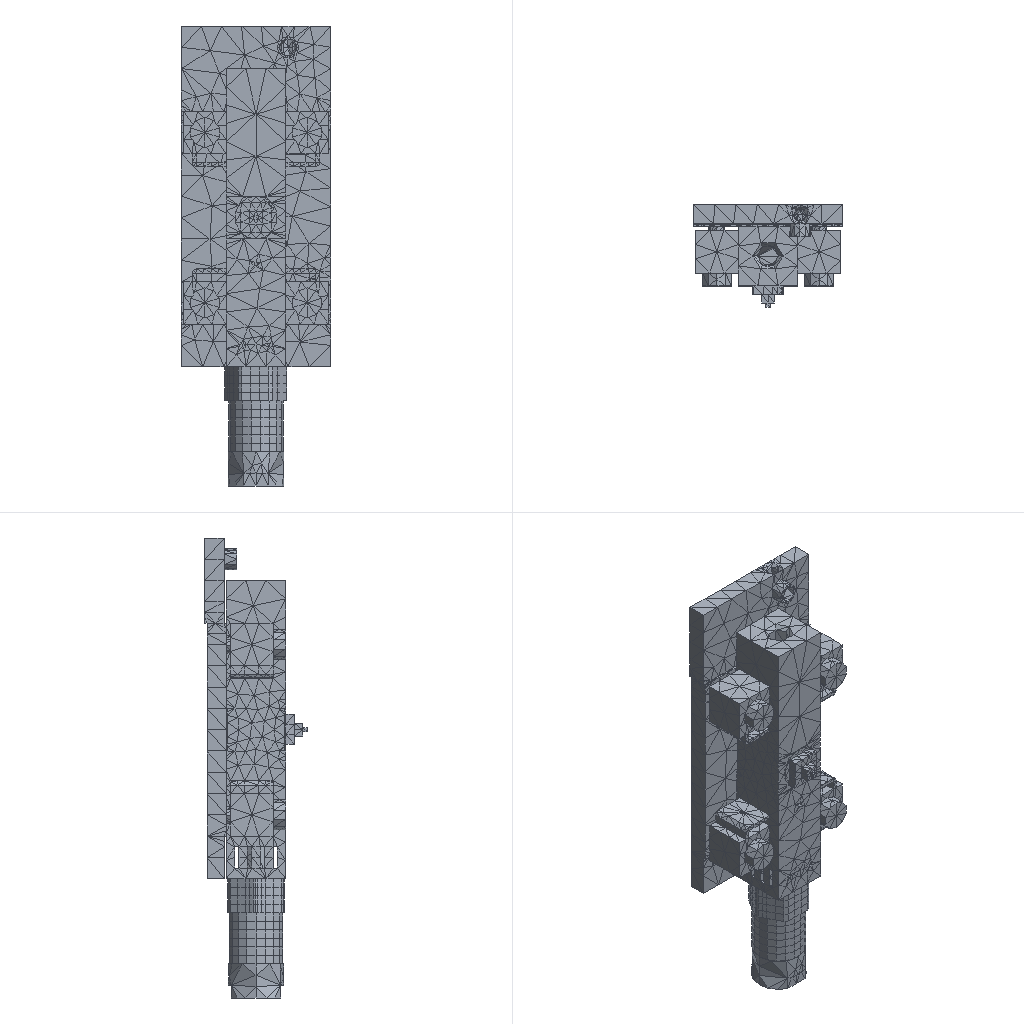Simulation study | ansys workbench
Ansys APDL input file, long lists of numbers shortened:
/batch
/config,noeldb,1     ! force off writing results to database
*get,_wallstrt,active,,time,wall
! ANSYS input file written by Workbench version 2022 R1
! File used for geometry attach: F:\ansys（分析文件汇总)\含底座模态分析\新建文件夹(4)\新建文件夹\完整版.STEP
/title,11111--__ (B5)
! ****** Begin Custom Load Command Snippet ******
/COM, ACT Extensions:
/COM,     LSDYNA, 2021.1
/COM,
! ****** End   Custom Load Command Snippet ******
*DIM,_wb_ProjectScratch_dir,string,248
_wb_ProjectScratch_dir(1) = 'F:\ansys（分析文件汇总)\含底座模态分析\_ProjectScratch\ScrD5D2\'
*DIM,_wb_SolverFiles_dir,string,248
_wb_SolverFiles_dir(1) = 'F:\ansys（分析文件汇总)\含底座模态分析\11111_files\dp0\SYS\MECH\'
*DIM,_wb_userfiles_dir,string,248
_wb_userfiles_dir(1) = 'F:\ansys（分析文件汇总)\含底座模态分析\11111_files\user_files\'
/com,--- Data in consistent NMM units. See Solving Units in the help system for more information.
/units,MPA
/nopr
/wb,file,start              !  signify a WB generated input file
/prep7
! Turn off shape checking because checks already performed inside WB mesher.
! See help system for more information.
SHPP,OFF,,NOWARN
/nolist
etcon,set             ! allow ANSYS to choose best KEYOP's for 180x elements, resets any applicable keyopt to MAPDL defaults
/com,*********** Nodes for the whole assembly ***********
nblock,3,,23060
(1i9,3e20.9e3)
        1    -7.593879241E+01     6.122424365E-01     1.555868903E+01
! (20963 more lines like these left out)
-1
/wb,elem,start            !  set before creation of elements
/com,*********** Elements for Body 1 "__|__-__6" ***********
et,1,187
eblock,19,solid,,4865
(19i9)
        1        1        1        1        0        0        0        0       10        0     2024     8034     8303     8491     8312    14700    15906    14703    14701
! (9729 more lines like these left out)
-1
/com,*********** Elements for Body 2 "___|__-__1" ***********
et,2,186
keyo,2,2,1          ! set full integration on SOLID186
eblock,19,solid,,35
(19i9)
        2        2        2        2        0        0        0        0       20        0      840     2544     2556     2561     2557     2579     2567     2562     2566
! (69 more lines like these left out)
-1
/com,*********** Elements for Body 3 "___|__-__1[2]" ***********
et,3,186
keyo,3,2,1          ! set full integration on SOLID186
eblock,19,solid,,35
(19i9)
        3        3        3        3        0        0        0        0       20        0      770     1924     1936     1941     1937     1959     1947     1942     1946
! (69 more lines like these left out)
-1
/com,*********** Elements for Body 4 "___|__-__1[3]" ***********
et,4,186
keyo,4,2,1          ! set full integration on SOLID186
eblock,19,solid,,35
(19i9)
        4        4        4        4        0        0        0        0       20        0      910     3164     3176     3181     3177     3199     3187     3182     3186
! (69 more lines like these left out)
-1
/com,*********** Elements for Body 5 "___|__-__1[4]" ***********
et,5,186
keyo,5,2,1          ! set full integration on SOLID186
eblock,19,solid,,35
(19i9)
        5        5        5        5        0        0        0        0       20        0      805     2234     2246     2251     2247     2269     2257     2252     2256
! (69 more lines like these left out)
-1
! (11 more sections like these left out)
/wb,elem,end               !  done creating elements
/com,*********** Send User Defined Coordinate System(s) ***********
csys,0
toffst,273.15,  ! Temperature offset from absolute zero
/com,*********** Set Reference Temperature ***********
tref,22.
/wb,mat,start              !  starting to send materials
/com,*********** Send Materials ***********
Temperature = 'TEMP' ! Temperature
TB,BISO,1,5,
TBTEMP,100
TBDATA,1,225,2091
TBTEMP,300
TBDATA,1,168,1577
TBTEMP,816
TBDATA,1,115,708
TBTEMP,1040
TBDATA,1,31,405
TBTEMP,1150
TBDATA,1,15,265
MPTEMP,,,,,,,,
MPTEMP,1,20
MPTEMP,2,100
MPTEMP,3,200
MPTEMP,4,300
MPTEMP,5,400
MPTEMP,6,500
MPTEMP,7,600
MPTEMP,8,700
MPTEMP,9,800
MPTEMP,10,900
MPTEMP,11,1000
MPTEMP,12,1100
MPTEMP,13,1200
MPDATA,EX,1, ,195000,191000,186000,180000,173000,164000,
MPDATA,EX,1, ,155000,144000,131000,117000,100000,81000,
MPDATA,EX,1, ,51000,	! tonne s^-2 mm^-1
MPTEMP,,,,,,,,
MPTEMP,,,,,,,,
MPTEMP,1,20
MPTEMP,2,100
MPTEMP,3,200
MPTEMP,4,300
MPTEMP,5,400
MPTEMP,6,500
MPTEMP,7,600
MPTEMP,8,700
MPTEMP,9,800
MPTEMP,10,900
MPTEMP,11,1000
MPTEMP,12,1100
MPTEMP,13,1200
MPDATA,NUXY,1, ,0.25,0.26,0.275,0.315,0.33,0.3,
MPDATA,NUXY,1, ,0.32,0.31,0.24,0.24,0.24,0.24,
MPDATA,NUXY,1, ,0.24,
MPTEMP,,,,,,,,
MPTEMP,,,,,,,,
MPTEMP,1,26.85
MPTEMP,2,126.85
MPTEMP,3,226.85
MPTEMP,4,326.85
MPTEMP,5,426.85
MPTEMP,6,526.85
MPTEMP,7,626.85
MPTEMP,8,726.85
MPTEMP,9,826.85
MPTEMP,10,926.85
MPTEMP,11,1026.85
MPTEMP,12,1126.85
MPTEMP,13,1226.85
MPTEMP,14,1326.85
MPTEMP,15,1426.85
MPTEMP,16,1526.85
MPTEMP,17,1626.85
MPTEMP,18,1726.85
MPTEMP,19,1826.85
MPTEMP,20,1926.85
MPTEMP,21,2026.85
MPTEMP,22,2126.85
MPTEMP,23,2226.85
MPTEMP,24,2326.85
MPTEMP,25,2426.85
MPTEMP,26,2526.85
MPTEMP,27,2626.85
MPTEMP,28,2726.85
MPDATA,DENS,1, ,7.954e-09,7.91e-09,7.864e-09,7.818e-09,7.771e-09,7.723e-09,
MPDATA,DENS,1, ,7.674e-09,7.624e-09,7.574e-09,7.523e-09,7.471e-09,7.419e-09,
! (1352 more lines like these left out)
/wb,mat,end                !  done sending materials
!************************* Model Summary ********************
!__|__-__6,	316不锈钢
,	matid,	1
!___|__-__1,	PZT-4,	matid,	2
!___|__-__1[2],	PZT-4,	matid,	3
!___|__-__1[3],	PZT-4,	matid,	4
!___|__-__1[4],	PZT-4,	matid,	5
!___|__-__1[5],	PZT-4,	matid,	6
!___|__-__1[6],	PZT-4,	matid,	7
!___|__1,	316不锈钢
,	matid,	8
!___|__1,	316不锈钢
,	matid,	9
!__|__-__5,	钨钢,	matid,	10
!__|__1,	316不锈钢
,	matid,	11
!__|__1,	316不锈钢
,	matid,	12
!__|__-__2,	316不锈钢
,	matid,	13
!__|__-__2[2],	316不锈钢
,	matid,	14
!__|__-__2[3],	316不锈钢
,	matid,	15
!__|__-__2[4],	316不锈钢
,	matid,	16
!************************* End Model Summary ********************
! get the diagonal of the bounding box. Needed later for other things
*get,_xmin,node,,mnloc,x
*get,_ymin,node,,mnloc,y
*get,_zmin,node,,mnloc,z
*get,_xmax,node,,mxloc,x
*get,_ymax,node,,mxloc,y
*get,_zmax,node,,mxloc,z
_ASMDIAG=(_xmax-_xmin)*(_xmax-_xmin)+(_ymax-_ymin)*(_ymax-_ymin)+(_zmax-_zmin)*(_zmax-_zmin)
_ASMDIAG=SQRT(_ASMDIAG)
/wb,contact,start          !  starting to send contact
/com,*********** Create Contact "接触区域" ***********
/com,            Real Constant Set For Above Contact Is 18 & 17
*set,tid,18
*set,cid,17
r,tid
r,cid
et,tid,170
et,cid,174
eblock,10,,,72
(15i9)
    15410       18       18       18        0     7091     7812     7209     7209     9306    10276     7209     9301
! (71 more lines like these left out)
-1
eblock,10,,,72
(15i9)
    15482       17       17       17        0     7091     7812     7209     7209     9306    10276     7209     9301
! (71 more lines like these left out)
-1
eblock,10,,,28
(15i9)
    15554       17       18       17        0        3        1        6        6      116      117        6      127
! (27 more lines like these left out)
-1
eblock,10,,,28
(15i9)
    15582       18       17       18        0        3        1        6        6      116      117        6      127
! (27 more lines like these left out)
-1
keyo,cid,8,2               ! auto create asymmetric contact (from Program Controlled setting)
keyo,cid,10,0              ! adjust contact stiffness each NR iteration (from Program Controlled setting)
keyo,cid,12,5              ! bonded always
keyo,cid,18,1              ! small sliding turned on by application
keyo,cid,2,0               ! augmented Lagrange (from Program Controlled setting)
keyo,cid,4,0               ! on Gauss point (from Program Controlled setting)
keyo,cid,9,1               ! ignore initial gaps/penetration
keyo,cid,7,0               ! No Prediction
rmod,tid,3,10.      ! FKN
rmod,tid,5,0.       ! ICONT
rmod,tid,6,0.       ! PINB
rmod,tid,10,0.      ! CNOF
rmod,tid,12,0.      ! FKT
rmod,tid,36,71      ! WB DSID
rmod,cid,3,10.      ! FKN
rmod,cid,5,0.       ! ICONT
rmod,cid,6,0.       ! PINB
rmod,cid,10,0.      ! CNOF
rmod,cid,12,0.      ! FKT
rmod,cid,36,71      ! WB DSID
/com,*********** Create Contact "接触区域 2" ***********
/com,            Real Constant Set For Above Contact Is 20 & 19
*set,tid,20
*set,cid,19
r,tid
r,cid
et,tid,170
et,cid,174
eblock,10,,,18
(15i9)
    15610       20       20       20        0     7098     7097     7481     7481     9356     9358     7481     9367
! (17 more lines like these left out)
-1
eblock,10,,,18
(15i9)
    15628       19       19       19        0     7098     7097     7481     7481     9356     9358     7481     9367
! (17 more lines like these left out)
-1
eblock,10,,,51
(15i9)
    15646       19       20       19        0     4333     4334     4550     4549     5009     5015     5426     5012
! (50 more lines like these left out)
-1
eblock,10,,,51
(15i9)
    15697       20       19       20        0     4333     4334     4550     4549     5009     5015     5426     5012
! (50 more lines like these left out)
-1
keyo,cid,8,2               ! auto create asymmetric contact (from Program Controlled setting)
keyo,cid,10,0              ! adjust contact stiffness each NR iteration (from Program Controlled setting)
keyo,cid,12,5              ! bonded always
keyo,cid,18,1              ! small sliding turned on by application
keyo,cid,2,0               ! augmented Lagrange (from Program Controlled setting)
keyo,cid,4,0               ! on Gauss point (from Program Controlled setting)
keyo,cid,9,1               ! ignore initial gaps/penetration
keyo,cid,7,0               ! No Prediction
rmod,tid,3,10.      ! FKN
rmod,tid,5,0.       ! ICONT
rmod,tid,6,0.       ! PINB
rmod,tid,10,0.      ! CNOF
rmod,tid,12,0.      ! FKT
rmod,tid,36,74      ! WB DSID
rmod,cid,3,10.      ! FKN
rmod,cid,5,0.       ! ICONT
rmod,cid,6,0.       ! PINB
rmod,cid,10,0.      ! CNOF
rmod,cid,12,0.      ! FKT
rmod,cid,36,74      ! WB DSID
/com,*********** Create Contact "接触区域 3" ***********
/com,            Real Constant Set For Above Contact Is 22 & 21
*set,tid,22
*set,cid,21
r,tid
r,cid
et,tid,170
et,cid,174
eblock,10,,,66
(15i9)
    15748       22       22       22        0     7771     7979     7048     7048    13698     8980     7048     8977
! (65 more lines like these left out)
-1
eblock,10,,,66
(15i9)
    15814       21       21       21        0     7771     7979     7048     7048    13698     8980     7048     8977
! (65 more lines like these left out)
-1
eblock,10,,,127
(15i9)
    15880       21       22       21        0     5467     5468     5596     5596     5886     5896     5596     5889
! (126 more lines like these left out)
-1
eblock,10,,,127
(15i9)
    16007       22       21       22        0     5467     5468     5596     5596     5886     5896     5596     5889
! (126 more lines like these left out)
-1
keyo,cid,8,2               ! auto create asymmetric contact (from Program Controlled setting)
keyo,cid,10,0              ! adjust contact stiffness each NR iteration (from Program Controlled setting)
keyo,cid,12,5              ! bonded always
keyo,cid,18,1              ! small sliding turned on by application
keyo,cid,2,0               ! augmented Lagrange (from Program Controlled setting)
keyo,cid,4,0               ! on Gauss point (from Program Controlled setting)
keyo,cid,9,1               ! ignore initial gaps/penetration
keyo,cid,7,0               ! No Prediction
rmod,tid,3,10.      ! FKN
rmod,tid,5,0.       ! ICONT
rmod,tid,6,0.       ! PINB
rmod,tid,10,0.      ! CNOF
rmod,tid,12,0.      ! FKT
rmod,tid,36,77      ! WB DSID
rmod,cid,3,10.      ! FKN
rmod,cid,5,0.       ! ICONT
rmod,cid,6,0.       ! PINB
rmod,cid,10,0.      ! CNOF
rmod,cid,12,0.      ! FKT
rmod,cid,36,77      ! WB DSID
/com,*********** Create Contact "接触区域 4" ***********
/com,            Real Constant Set For Above Contact Is 24 & 23
*set,tid,24
*set,cid,23
r,tid
r,cid
et,tid,170
et,cid,174
eblock,10,,,24
(15i9)
    16134       24       24       24        0     7044     7881     7498     7498     8932    12249     7498     8929
! (23 more lines like these left out)
-1
eblock,10,,,24
(15i9)
    16158       23       23       23        0     7044     7881     7498     7498     8932    12249     7498     8929
! (23 more lines like these left out)
-1
eblock,10,,,36
(15i9)
    16182       23       24       23        0     3540     3541     3569     3569     3910     3915     3569     3912
! (35 more lines like these left out)
-1
eblock,10,,,36
(15i9)
    16218       24       23       24        0     3540     3541     3569     3569     3910     3915     3569     3912
! (35 more lines like these left out)
-1
keyo,cid,8,2               ! auto create asymmetric contact (from Program Controlled setting)
keyo,cid,10,0              ! adjust contact stiffness each NR iteration (from Program Controlled setting)
keyo,cid,12,5              ! bonded always
keyo,cid,18,1              ! small sliding turned on by application
keyo,cid,2,0               ! augmented Lagrange (from Program Controlled setting)
keyo,cid,4,0               ! on Gauss point (from Program Controlled setting)
keyo,cid,9,1               ! ignore initial gaps/penetration
keyo,cid,7,0               ! No Prediction
rmod,tid,3,10.      ! FKN
rmod,tid,5,0.       ! ICONT
rmod,tid,6,0.       ! PINB
rmod,tid,10,0.      ! CNOF
rmod,tid,12,0.      ! FKT
rmod,tid,36,80      ! WB DSID
rmod,cid,3,10.      ! FKN
rmod,cid,5,0.       ! ICONT
rmod,cid,6,0.       ! PINB
rmod,cid,10,0.      ! CNOF
rmod,cid,12,0.      ! FKT
rmod,cid,36,80      ! WB DSID
/com,*********** Create Contact "接触区域 5" ***********
/com,            Real Constant Set For Above Contact Is 26 & 25
*set,tid,26
*set,cid,25
r,tid
r,cid
et,tid,170
et,cid,174
eblock,10,,,200
(15i9)
    16254       26       26       26        0     8149     8178     8152     8152    15277    15300     8152    15274
! (199 more lines like these left out)
-1
eblock,10,,,200
(15i9)
    16454       25       25       25        0     8149     8178     8152     8152    15277    15300     8152    15274
! (199 more lines like these left out)
-1
eblock,10,,,158
(15i9)
    16654       25       26       25        0    16812    16862    16828    16828    20339    20448    16828    20337
! (157 more lines like these left out)
-1
eblock,10,,,158
(15i9)
    16812       26       25       26        0    16812    16862    16828    16828    20339    20448    16828    20337
! (157 more lines like these left out)
-1
keyo,cid,8,2               ! auto create asymmetric contact (from Program Controlled setting)
keyo,cid,10,0              ! adjust contact stiffness each NR iteration (from Program Controlled setting)
keyo,cid,12,5              ! bonded always
keyo,cid,18,1              ! small sliding turned on by application
keyo,cid,2,0               ! augmented Lagrange (from Program Controlled setting)
keyo,cid,4,0               ! on Gauss point (from Program Controlled setting)
keyo,cid,9,1               ! ignore initial gaps/penetration
keyo,cid,7,0               ! No Prediction
rmod,tid,3,10.      ! FKN
rmod,tid,5,0.       ! ICONT
rmod,tid,6,0.       ! PINB
rmod,tid,10,0.      ! CNOF
rmod,tid,12,0.      ! FKT
rmod,tid,36,83      ! WB DSID
rmod,cid,3,10.      ! FKN
rmod,cid,5,0.       ! ICONT
rmod,cid,6,0.       ! PINB
rmod,cid,10,0.      ! CNOF
rmod,cid,12,0.      ! FKT
rmod,cid,36,83      ! WB DSID
! (18 more sections like these left out)
/wb,contact,end            !  done creating contacts
/golist
/wb,load,start             !  starting to send loads
/com,*********** Fixed Supports ***********
CMBLOCK,_FIXEDSU,NODE,     1547
(8i10)
       639       640       641       642       643       644       645       646
! (193 more lines like these left out)
cmsel,s,_FIXEDSU
d,all,all
nsel,all
/gst,on,on
fini
*get,_numnode,node,0,count
*get,_numelem,elem,0,count
*get, _MAXELEMNUM, elem, 0, NUM, MAX
*get, _MAXNODENUM, node, 0, NUM, MAX
*get, _MAXELEMTYPE, etyp, 0, NUM, MAX
*get, _MAXREALCONST, real, 0, NUM, MAX
/go
/wb,load,end               !  done creating loads
/com,--- Number of total nodes = %_numnode%
/com,--- Number of contact elements = 4058
/com,--- Number of spring elements = 0
/com,--- Number of bearing elements = 0
/com,--- Number of solid elements = 9315
/com,--- Number of condensed parts = 0
/com,--- Number of total elements = %_numelem%
*get,_wallbsol,active,,time,wall
/solu
antype,2                   ! modal analysis
_thickRatio=0.313   ! Ratio of thick parts in the model
modopt,lanb,6,50000.,70000.
outres,erase
outres,all,none
outres,nsol,all
outres,etmp,all
mxpand                    ! default expand in case of complex solution
dmpopt,esav,no
dmpopt,emat,no
dmpopt,full,no
! *********** WB SOLVE COMMAND ***********
! check interactive state
*get,ANSINTER_,active,,int
*if,ANSINTER_,ne,0,then
/eof
*endif
solve
/com *************** Write FE CONNECTORS *********
CEWRITE,file,ce,,INTE
*get,_nmodalsolproc,active,0,numcpu
fini
/nopr
*get,_numnode,node,0,count
*get,_numelem,elem,0,count
*get, _MAXELEMNUM, elem, 0, NUM, MAX
*get, _MAXNODENUM, node, 0, NUM, MAX,,,INTERNAL
*get, _MAXELEMTYPE, etyp, 0, NUM, MAX
*get, _MAXREALCONST, real, 0, NUM, MAX
/gopr
*get,_wallasol,active,,time,wall
/post1
/nopr
*dim,_direction,CHAR,6,1
_direction(1) = 'X'
_direction(2) = 'Y'
_direction(3) = 'Z'
_direction(4) = 'ROTX'
_direction(5) = 'ROTY'
_direction(6) = 'ROTZ'
*get,_lastLS,active,0,set,LSTP
*get,_beginset,active,0,set,nset,first,_lastLS
*get,_endset,active,0,set,nset,last,_lastLS
_nummodes = 0
*if,_endset,gt,0,then
_nummodes = _endset - _beginset + 1
*endif
*do,i_mode,1,_nummodes
   *do,j_component,1,6
			*get,PFACT_%i_mode%_%j_component%,MODE,%i_mode%,PFACT,,DIREC,_direction(%j_component%)
   *enddo
*enddo
*dim,_tmdirection,CHAR,6,1
_tmdirection(1) = 'X'
_tmdirection(2) = 'Y'
_tmdirection(3) = 'Z'
_tmdirection(4) = 'X'
_tmdirection(5) = 'Y'
_tmdirection(6) = 'Z'
*do,j_component,1,6
    *if,j_component,gt,3,then
        *get,TOTALMASS_%j_component%,ELEM,0,IOR,_tmdirection(%j_component%)
    *else
        *get,TOTALMASS_%j_component%,ELEM,0,MTOT,_tmdirection(%j_component%)
    *endif
*enddo
/gopr
xmlo,ENCODING,ISO-8859-1
xmlo,parm
/xml,parm,xml
fini
/gopr
*get,_walldone,active,,time,wall
_preptime=(_wallbsol-_wallstrt)*3600
_solvtime=(_wallasol-_wallbsol)*3600
_posttime=(_walldone-_wallasol)*3600
_totaltim=(_walldone-_wallstrt)*3600
*get,_dlbratio,active,0,solu,dlbr
*get,_combtime,active,0,solu,comb
*get,_ssmode,active,0,solu,ssmm
*get,_ndofs,active,0,solu,ndof
/fclean				!clean distributed files
/com,--- Total number of nodes = %_numnode%
/com,--- Total number of elements = %_numelem%
/com,--- Element load balance ratio = %_dlbratio%
/com,--- Time to combine distributed files = %_combtime%
/com,--- Sparse memory mode = %_ssmode%
/com,--- Number of DOF = %_ndofs%
/wb,file,end               ! done with WB generated input